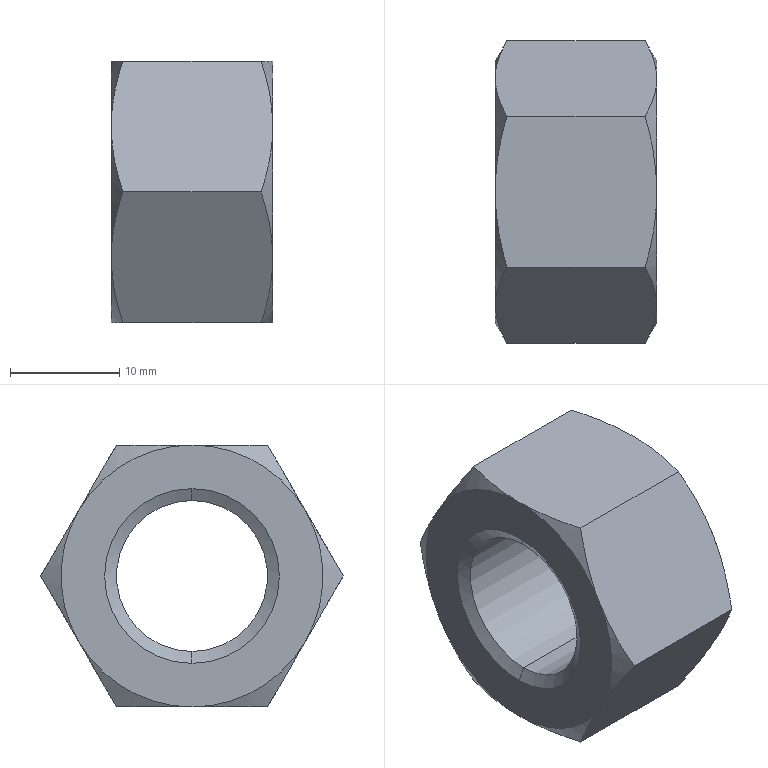Part | SolidWorks | features BaseBody 1 | 1 solid | 26 faces | box 14.8 x 27.713 x 24 mm | volume 5097 mm3 | cone 16 | plane 8 | cylinder 2 | commonest cylinder face diameters 13.835 x2
STEP:
#1=CARTESIAN_POINT('',(0.625,0.,6.918));
#2=VERTEX_POINT('',#1);
#3=CARTESIAN_POINT('',(0.625,0.,-6.918));
#4=VERTEX_POINT('',#3);
#5=CARTESIAN_POINT('',(0.625,0.,0.));
#6=DIRECTION('',(1.,0.,0.));
#7=DIRECTION('',(0.,0.,-1.));
#8=AXIS2_PLACEMENT_3D('',#5,#6,#7);
#9=CIRCLE('',#8,6.918);
#10=EDGE_CURVE('',#2,#4,#9,.T.);
#11=ORIENTED_EDGE('',*,*,#10,.F.);
#12=CARTESIAN_POINT('',(14.175,0.,6.918));
#13=VERTEX_POINT('',#12);
#14=CARTESIAN_POINT('',(-24.735,0.,6.918));
#15=DIRECTION('',(1.,0.,0.));
#16=VECTOR('',#15,1000.);
#17=LINE('',#14,#16);
#18=EDGE_CURVE('',#2,#13,#17,.T.);
#19=ORIENTED_EDGE('',*,*,#18,.T.);
#20=CARTESIAN_POINT('',(14.175,0.,-6.918));
#21=VERTEX_POINT('',#20);
#22=CARTESIAN_POINT('',(14.175,0.,0.));
#23=DIRECTION('',(-1.,0.,0.));
#24=DIRECTION('',(0.,0.,-1.));
#25=AXIS2_PLACEMENT_3D('',#22,#23,#24);
#26=CIRCLE('',#25,6.918);
#27=EDGE_CURVE('',#21,#13,#26,.T.);
#28=ORIENTED_EDGE('',*,*,#27,.F.);
#29=CARTESIAN_POINT('',(-24.735,0.,-6.918));
#30=DIRECTION('',(1.,0.,0.));
#31=VECTOR('',#30,1000.);
#32=LINE('',#29,#31);
#33=EDGE_CURVE('',#4,#21,#32,.T.);
#34=ORIENTED_EDGE('',*,*,#33,.F.);
#35=EDGE_LOOP('',(#11,#19,#28,#34));
#36=FACE_OUTER_BOUND('',#35,.T.);
#37=CARTESIAN_POINT('',(-24.735,0.,0.));
#38=DIRECTION('',(1.,0.,0.));
#39=DIRECTION('',(0.,0.,-1.));
#40=AXIS2_PLACEMENT_3D('',#37,#38,#39);
#41=CYLINDRICAL_SURFACE('',#40,6.918);
#42=ADVANCED_FACE('',(#36),#41,.F.);
#43=ORIENTED_EDGE('',*,*,#10,.T.);
#44=CARTESIAN_POINT('',(0.,0.,-8.));
#45=VERTEX_POINT('',#44);
#46=CARTESIAN_POINT('',(0.,0.,-8.));
#47=DIRECTION('',(-0.5,0.,-0.866));
#48=VECTOR('',#47,1000.);
#49=LINE('',#46,#48);
#50=EDGE_CURVE('',#4,#45,#49,.T.);
#51=ORIENTED_EDGE('',*,*,#50,.T.);
#52=CARTESIAN_POINT('',(0.,0.,8.));
#53=VERTEX_POINT('',#52);
#54=CARTESIAN_POINT('',(0.,0.,0.));
#55=DIRECTION('',(1.,0.,0.));
#56=DIRECTION('',(0.,0.,1.));
#57=AXIS2_PLACEMENT_3D('',#54,#55,#56);
#58=CIRCLE('',#57,8.);
#59=EDGE_CURVE('',#53,#45,#58,.T.);
#60=ORIENTED_EDGE('',*,*,#59,.F.);
#61=CARTESIAN_POINT('',(0.,0.,8.));
#62=DIRECTION('',(-0.5,0.,0.866));
#63=VECTOR('',#62,1000.);
#64=LINE('',#61,#63);
#65=EDGE_CURVE('',#2,#53,#64,.T.);
#66=ORIENTED_EDGE('',*,*,#65,.F.);
#67=EDGE_LOOP('',(#43,#51,#60,#66));
#68=FACE_OUTER_BOUND('',#67,.T.);
#69=CARTESIAN_POINT('',(0.,0.,0.));
#70=DIRECTION('',(-1.,0.,0.));
#71=DIRECTION('',(0.,0.,1.));
#72=AXIS2_PLACEMENT_3D('',#69,#70,#71);
#73=CONICAL_SURFACE('',#72,8.,1.047);
#74=ADVANCED_FACE('',(#68),#73,.F.);
#75=ORIENTED_EDGE('',*,*,#27,.T.);
#76=CARTESIAN_POINT('',(14.8,0.,8.));
#77=VERTEX_POINT('',#76);
#78=CARTESIAN_POINT('',(14.8,0.,8.));
#79=DIRECTION('',(0.5,0.,0.866));
#80=VECTOR('',#79,1000.);
#81=LINE('',#78,#80);
#82=EDGE_CURVE('',#13,#77,#81,.T.);
#83=ORIENTED_EDGE('',*,*,#82,.T.);
#84=CARTESIAN_POINT('',(14.8,0.,-8.));
#85=VERTEX_POINT('',#84);
#86=CARTESIAN_POINT('',(14.8,0.,0.));
#87=DIRECTION('',(-1.,0.,0.));
#88=DIRECTION('',(0.,0.,-1.));
#89=AXIS2_PLACEMENT_3D('',#86,#87,#88);
#90=CIRCLE('',#89,8.);
#91=EDGE_CURVE('',#85,#77,#90,.T.);
#92=ORIENTED_EDGE('',*,*,#91,.F.);
#93=CARTESIAN_POINT('',(14.8,0.,-8.));
#94=DIRECTION('',(0.5,0.,-0.866));
#95=VECTOR('',#94,1000.);
#96=LINE('',#93,#95);
#97=EDGE_CURVE('',#21,#85,#96,.T.);
#98=ORIENTED_EDGE('',*,*,#97,.F.);
#99=EDGE_LOOP('',(#75,#83,#92,#98));
#100=FACE_OUTER_BOUND('',#99,.T.);
#101=CARTESIAN_POINT('',(14.8,0.,0.));
#102=DIRECTION('',(1.,0.,0.));
#103=DIRECTION('',(0.,0.,-1.));
#104=AXIS2_PLACEMENT_3D('',#101,#102,#103);
#105=CONICAL_SURFACE('',#104,8.,1.047);
#106=ADVANCED_FACE('',(#100),#105,.F.);
#107=ORIENTED_EDGE('',*,*,#18,.F.);
#108=CARTESIAN_POINT('',(0.625,0.,0.));
#109=DIRECTION('',(1.,0.,0.));
#110=DIRECTION('',(0.,0.,-1.));
#111=AXIS2_PLACEMENT_3D('',#108,#109,#110);
#112=CIRCLE('',#111,6.918);
#113=EDGE_CURVE('',#4,#2,#112,.T.);
#114=ORIENTED_EDGE('',*,*,#113,.F.);
#115=ORIENTED_EDGE('',*,*,#33,.T.);
#116=CARTESIAN_POINT('',(14.175,0.,0.));
#117=DIRECTION('',(-1.,0.,0.));
#118=DIRECTION('',(0.,0.,-1.));
#119=AXIS2_PLACEMENT_3D('',#116,#117,#118);
#120=CIRCLE('',#119,6.918);
#121=EDGE_CURVE('',#13,#21,#120,.T.);
#122=ORIENTED_EDGE('',*,*,#121,.F.);
#123=EDGE_LOOP('',(#107,#114,#115,#122));
#124=FACE_OUTER_BOUND('',#123,.T.);
#125=CARTESIAN_POINT('',(-24.735,0.,0.));
#126=DIRECTION('',(1.,0.,0.));
#127=DIRECTION('',(0.,0.,-1.));
#128=AXIS2_PLACEMENT_3D('',#125,#126,#127);
#129=CYLINDRICAL_SURFACE('',#128,6.918);
#130=ADVANCED_FACE('',(#124),#129,.F.);
#131=ORIENTED_EDGE('',*,*,#50,.F.);
#132=ORIENTED_EDGE('',*,*,#113,.T.);
#133=ORIENTED_EDGE('',*,*,#65,.T.);
#134=CARTESIAN_POINT('',(0.,0.,0.));
#135=DIRECTION('',(1.,0.,0.));
#136=DIRECTION('',(0.,0.,1.));
#137=AXIS2_PLACEMENT_3D('',#134,#135,#136);
#138=CIRCLE('',#137,8.);
#139=EDGE_CURVE('',#45,#53,#138,.T.);
#140=ORIENTED_EDGE('',*,*,#139,.F.);
#141=EDGE_LOOP('',(#131,#132,#133,#140));
#142=FACE_OUTER_BOUND('',#141,.T.);
#143=CARTESIAN_POINT('',(0.,0.,0.));
#144=DIRECTION('',(-1.,0.,0.));
#145=DIRECTION('',(0.,0.,1.));
#146=AXIS2_PLACEMENT_3D('',#143,#144,#145);
#147=CONICAL_SURFACE('',#146,8.,1.047);
#148=ADVANCED_FACE('',(#142),#147,.F.);
#149=ORIENTED_EDGE('',*,*,#82,.F.);
#150=ORIENTED_EDGE('',*,*,#121,.T.);
#151=ORIENTED_EDGE('',*,*,#97,.T.);
#152=CARTESIAN_POINT('',(14.8,0.,0.));
#153=DIRECTION('',(-1.,0.,0.));
#154=DIRECTION('',(0.,0.,-1.));
#155=AXIS2_PLACEMENT_3D('',#152,#153,#154);
#156=CIRCLE('',#155,8.);
#157=EDGE_CURVE('',#77,#85,#156,.T.);
#158=ORIENTED_EDGE('',*,*,#157,.F.);
#159=EDGE_LOOP('',(#149,#150,#151,#158));
#160=FACE_OUTER_BOUND('',#159,.T.);
#161=CARTESIAN_POINT('',(14.8,0.,0.));
#162=DIRECTION('',(1.,0.,0.));
#163=DIRECTION('',(0.,0.,-1.));
#164=AXIS2_PLACEMENT_3D('',#161,#162,#163);
#165=CONICAL_SURFACE('',#164,8.,1.047);
#166=ADVANCED_FACE('',(#160),#165,.F.);
#167=ORIENTED_EDGE('',*,*,#59,.T.);
#168=ORIENTED_EDGE('',*,*,#139,.T.);
#169=EDGE_LOOP('',(#167,#168));
#170=FACE_BOUND('',#169,.T.);
#171=CARTESIAN_POINT('',(0.,0.,12.));
#172=VERTEX_POINT('',#171);
#173=CARTESIAN_POINT('',(0.,-10.392,6.));
#174=VERTEX_POINT('',#173);
#175=CARTESIAN_POINT('',(0.,0.,0.));
#176=DIRECTION('',(1.,0.,0.));
#177=DIRECTION('',(0.,0.,-1.));
#178=AXIS2_PLACEMENT_3D('',#175,#176,#177);
#179=CIRCLE('',#178,12.);
#180=EDGE_CURVE('',#172,#174,#179,.T.);
#181=ORIENTED_EDGE('',*,*,#180,.F.);
#182=CARTESIAN_POINT('',(0.,10.392,6.));
#183=VERTEX_POINT('',#182);
#184=CARTESIAN_POINT('',(0.,0.,0.));
#185=DIRECTION('',(1.,0.,0.));
#186=DIRECTION('',(0.,0.,-1.));
#187=AXIS2_PLACEMENT_3D('',#184,#185,#186);
#188=CIRCLE('',#187,12.);
#189=EDGE_CURVE('',#183,#172,#188,.T.);
#190=ORIENTED_EDGE('',*,*,#189,.F.);
#191=CARTESIAN_POINT('',(0.,10.392,-6.));
#192=VERTEX_POINT('',#191);
#193=CARTESIAN_POINT('',(0.,0.,0.));
#194=DIRECTION('',(1.,0.,0.));
#195=DIRECTION('',(0.,0.,-1.));
#196=AXIS2_PLACEMENT_3D('',#193,#194,#195);
#197=CIRCLE('',#196,12.);
#198=EDGE_CURVE('',#192,#183,#197,.T.);
#199=ORIENTED_EDGE('',*,*,#198,.F.);
#200=CARTESIAN_POINT('',(0.,0.,-12.));
#201=VERTEX_POINT('',#200);
#202=CARTESIAN_POINT('',(0.,0.,0.));
#203=DIRECTION('',(1.,0.,0.));
#204=DIRECTION('',(0.,0.,-1.));
#205=AXIS2_PLACEMENT_3D('',#202,#203,#204);
#206=CIRCLE('',#205,12.);
#207=EDGE_CURVE('',#201,#192,#206,.T.);
#208=ORIENTED_EDGE('',*,*,#207,.F.);
#209=CARTESIAN_POINT('',(0.,-10.392,-6.));
#210=VERTEX_POINT('',#209);
#211=CARTESIAN_POINT('',(0.,0.,0.));
#212=DIRECTION('',(1.,0.,0.));
#213=DIRECTION('',(0.,0.,-1.));
#214=AXIS2_PLACEMENT_3D('',#211,#212,#213);
#215=CIRCLE('',#214,12.);
#216=EDGE_CURVE('',#210,#201,#215,.T.);
#217=ORIENTED_EDGE('',*,*,#216,.F.);
#218=CARTESIAN_POINT('',(0.,0.,0.));
#219=DIRECTION('',(1.,0.,0.));
#220=DIRECTION('',(0.,0.,-1.));
#221=AXIS2_PLACEMENT_3D('',#218,#219,#220);
#222=CIRCLE('',#221,12.);
#223=EDGE_CURVE('',#174,#210,#222,.T.);
#224=ORIENTED_EDGE('',*,*,#223,.F.);
#225=EDGE_LOOP('',(#181,#190,#199,#208,#217,#224));
#226=FACE_OUTER_BOUND('',#225,.T.);
#227=CARTESIAN_POINT('',(0.,0.,0.));
#228=DIRECTION('',(1.,0.,0.));
#229=DIRECTION('',(0.,0.,-1.));
#230=AXIS2_PLACEMENT_3D('',#227,#228,#229);
#231=PLANE('',#230);
#232=ADVANCED_FACE('',(#170,#226),#231,.F.);
#233=ORIENTED_EDGE('',*,*,#91,.T.);
#234=ORIENTED_EDGE('',*,*,#157,.T.);
#235=EDGE_LOOP('',(#233,#234));
#236=FACE_BOUND('',#235,.T.);
#237=CARTESIAN_POINT('',(14.8,0.,12.));
#238=VERTEX_POINT('',#237);
#239=CARTESIAN_POINT('',(14.8,-10.392,6.));
#240=VERTEX_POINT('',#239);
#241=CARTESIAN_POINT('',(14.8,0.,0.));
#242=DIRECTION('',(1.,0.,0.));
#243=DIRECTION('',(0.,0.,1.));
#244=AXIS2_PLACEMENT_3D('',#241,#242,#243);
#245=CIRCLE('',#244,12.);
#246=EDGE_CURVE('',#238,#240,#245,.T.);
#247=ORIENTED_EDGE('',*,*,#246,.T.);
#248=CARTESIAN_POINT('',(14.8,-10.392,-6.));
#249=VERTEX_POINT('',#248);
#250=CARTESIAN_POINT('',(14.8,0.,0.));
#251=DIRECTION('',(1.,0.,0.));
#252=DIRECTION('',(0.,0.,1.));
#253=AXIS2_PLACEMENT_3D('',#250,#251,#252);
#254=CIRCLE('',#253,12.);
#255=EDGE_CURVE('',#240,#249,#254,.T.);
#256=ORIENTED_EDGE('',*,*,#255,.T.);
#257=CARTESIAN_POINT('',(14.8,0.,-12.));
#258=VERTEX_POINT('',#257);
#259=CARTESIAN_POINT('',(14.8,0.,0.));
#260=DIRECTION('',(1.,0.,0.));
#261=DIRECTION('',(0.,0.,1.));
#262=AXIS2_PLACEMENT_3D('',#259,#260,#261);
#263=CIRCLE('',#262,12.);
#264=EDGE_CURVE('',#249,#258,#263,.T.);
#265=ORIENTED_EDGE('',*,*,#264,.T.);
#266=CARTESIAN_POINT('',(14.8,10.392,-6.));
#267=VERTEX_POINT('',#266);
#268=CARTESIAN_POINT('',(14.8,0.,0.));
#269=DIRECTION('',(1.,0.,0.));
#270=DIRECTION('',(0.,0.,1.));
#271=AXIS2_PLACEMENT_3D('',#268,#269,#270);
#272=CIRCLE('',#271,12.);
#273=EDGE_CURVE('',#258,#267,#272,.T.);
#274=ORIENTED_EDGE('',*,*,#273,.T.);
#275=CARTESIAN_POINT('',(14.8,10.392,6.));
#276=VERTEX_POINT('',#275);
#277=CARTESIAN_POINT('',(14.8,0.,0.));
#278=DIRECTION('',(1.,0.,0.));
#279=DIRECTION('',(0.,0.,1.));
#280=AXIS2_PLACEMENT_3D('',#277,#278,#279);
#281=CIRCLE('',#280,12.);
#282=EDGE_CURVE('',#267,#276,#281,.T.);
#283=ORIENTED_EDGE('',*,*,#282,.T.);
#284=CARTESIAN_POINT('',(14.8,0.,0.));
#285=DIRECTION('',(1.,0.,0.));
#286=DIRECTION('',(0.,0.,1.));
#287=AXIS2_PLACEMENT_3D('',#284,#285,#286);
#288=CIRCLE('',#287,12.);
#289=EDGE_CURVE('',#276,#238,#288,.T.);
#290=ORIENTED_EDGE('',*,*,#289,.T.);
#291=EDGE_LOOP('',(#247,#256,#265,#274,#283,#290));
#292=FACE_OUTER_BOUND('',#291,.T.);
#293=CARTESIAN_POINT('',(14.8,0.,0.));
#294=DIRECTION('',(1.,0.,0.));
#295=DIRECTION('',(0.,0.,-1.));
#296=AXIS2_PLACEMENT_3D('',#293,#294,#295);
#297=PLANE('',#296);
#298=ADVANCED_FACE('',(#236,#292),#297,.T.);
#299=ORIENTED_EDGE('',*,*,#223,.T.);
#300=CARTESIAN_POINT('',(1.072,-13.856,0.000000014));
#301=VERTEX_POINT('',#300);
#302=CARTESIAN_POINT('',(0.,-10.392,-6.));
#303=CARTESIAN_POINT('',(0.,-10.983,-4.976));
#304=CARTESIAN_POINT('',(0.1025,-11.567,-3.966));
#305=CARTESIAN_POINT('',(0.4756,-12.72,-1.968));
#306=CARTESIAN_POINT('',(0.7451,-13.291,-0.9802));
#307=CARTESIAN_POINT('',(1.072,-13.856,0.000000014));
#308=B_SPLINE_CURVE_WITH_KNOTS('',3,(#302,#303,#304,#305,#306,#307),.UNSPECIFIED.,.F.,.F.,(4,2,4),(0.,0.003505,0.007011),.UNSPECIFIED.);
#309=EDGE_CURVE('',#210,#301,#308,.T.);
#310=ORIENTED_EDGE('',*,*,#309,.T.);
#311=CARTESIAN_POINT('',(1.072,-13.856,0.000000014));
#312=CARTESIAN_POINT('',(0.7451,-13.291,0.9802));
#313=CARTESIAN_POINT('',(0.4756,-12.72,1.968));
#314=CARTESIAN_POINT('',(0.1025,-11.567,3.966));
#315=CARTESIAN_POINT('',(0.,-10.983,4.976));
#316=CARTESIAN_POINT('',(0.,-10.392,6.));
#317=B_SPLINE_CURVE_WITH_KNOTS('',3,(#311,#312,#313,#314,#315,#316),.UNSPECIFIED.,.F.,.F.,(4,2,4),(0.,0.003505,0.007011),.UNSPECIFIED.);
#318=EDGE_CURVE('',#301,#174,#317,.T.);
#319=ORIENTED_EDGE('',*,*,#318,.T.);
#320=EDGE_LOOP('',(#299,#310,#319));
#321=FACE_OUTER_BOUND('',#320,.T.);
#322=CARTESIAN_POINT('',(1.078,0.,0.));
#323=DIRECTION('',(1.,0.,0.));
#324=DIRECTION('',(0.,0.,-1.));
#325=AXIS2_PLACEMENT_3D('',#322,#323,#324);
#326=CONICAL_SURFACE('',#325,13.868,1.047);
#327=ADVANCED_FACE('',(#321),#326,.T.);
#328=ORIENTED_EDGE('',*,*,#180,.T.);
#329=CARTESIAN_POINT('',(1.072,-6.928,12.));
#330=VERTEX_POINT('',#329);
#331=CARTESIAN_POINT('',(0.,-10.392,6.));
#332=CARTESIAN_POINT('',(0.,-9.801,7.024));
#333=CARTESIAN_POINT('',(0.1025,-9.218,8.034));
#334=CARTESIAN_POINT('',(0.4756,-8.064,10.032));
#335=CARTESIAN_POINT('',(0.7451,-7.494,11.02));
#336=CARTESIAN_POINT('',(1.072,-6.928,12.));
#337=B_SPLINE_CURVE_WITH_KNOTS('',3,(#331,#332,#333,#334,#335,#336),.UNSPECIFIED.,.F.,.F.,(4,2,4),(0.,0.003505,0.007011),.UNSPECIFIED.);
#338=EDGE_CURVE('',#174,#330,#337,.T.);
#339=ORIENTED_EDGE('',*,*,#338,.T.);
#340=CARTESIAN_POINT('',(1.072,-6.928,12.));
#341=CARTESIAN_POINT('',(0.7451,-5.796,12.));
#342=CARTESIAN_POINT('',(0.4756,-4.656,12.));
#343=CARTESIAN_POINT('',(0.1025,-2.349,12.));
#344=CARTESIAN_POINT('',(0.,-1.182,12.));
#345=CARTESIAN_POINT('',(0.,0.,12.));
#346=B_SPLINE_CURVE_WITH_KNOTS('',3,(#340,#341,#342,#343,#344,#345),.UNSPECIFIED.,.F.,.F.,(4,2,4),(0.,0.003505,0.007011),.UNSPECIFIED.);
#347=EDGE_CURVE('',#330,#172,#346,.T.);
#348=ORIENTED_EDGE('',*,*,#347,.T.);
#349=EDGE_LOOP('',(#328,#339,#348));
#350=FACE_OUTER_BOUND('',#349,.T.);
#351=CARTESIAN_POINT('',(1.078,0.,0.));
#352=DIRECTION('',(1.,0.,0.));
#353=DIRECTION('',(0.,0.,-1.));
#354=AXIS2_PLACEMENT_3D('',#351,#352,#353);
#355=CONICAL_SURFACE('',#354,13.868,1.047);
#356=ADVANCED_FACE('',(#350),#355,.T.);
#357=ORIENTED_EDGE('',*,*,#189,.T.);
#358=CARTESIAN_POINT('',(1.072,6.928,12.));
#359=VERTEX_POINT('',#358);
#360=CARTESIAN_POINT('',(0.,0.,12.));
#361=CARTESIAN_POINT('',(0.,1.182,12.));
#362=CARTESIAN_POINT('',(0.1025,2.349,12.));
#363=CARTESIAN_POINT('',(0.4756,4.656,12.));
#364=CARTESIAN_POINT('',(0.7451,5.796,12.));
#365=CARTESIAN_POINT('',(1.072,6.928,12.));
#366=B_SPLINE_CURVE_WITH_KNOTS('',3,(#360,#361,#362,#363,#364,#365),.UNSPECIFIED.,.F.,.F.,(4,2,4),(0.,0.003505,0.007011),.UNSPECIFIED.);
#367=EDGE_CURVE('',#172,#359,#366,.T.);
#368=ORIENTED_EDGE('',*,*,#367,.T.);
#369=CARTESIAN_POINT('',(1.072,6.928,12.));
#370=CARTESIAN_POINT('',(0.7451,7.494,11.02));
#371=CARTESIAN_POINT('',(0.4756,8.064,10.032));
#372=CARTESIAN_POINT('',(0.1025,9.218,8.034));
#373=CARTESIAN_POINT('',(0.,9.801,7.024));
#374=CARTESIAN_POINT('',(0.,10.392,6.));
#375=B_SPLINE_CURVE_WITH_KNOTS('',3,(#369,#370,#371,#372,#373,#374),.UNSPECIFIED.,.F.,.F.,(4,2,4),(0.,0.003505,0.007011),.UNSPECIFIED.);
#376=EDGE_CURVE('',#359,#183,#375,.T.);
#377=ORIENTED_EDGE('',*,*,#376,.T.);
#378=EDGE_LOOP('',(#357,#368,#377));
#379=FACE_OUTER_BOUND('',#378,.T.);
#380=CARTESIAN_POINT('',(1.078,0.,0.));
#381=DIRECTION('',(1.,0.,0.));
#382=DIRECTION('',(0.,0.,-1.));
#383=AXIS2_PLACEMENT_3D('',#380,#381,#382);
#384=CONICAL_SURFACE('',#383,13.868,1.047);
#385=ADVANCED_FACE('',(#379),#384,.T.);
#386=ORIENTED_EDGE('',*,*,#198,.T.);
#387=CARTESIAN_POINT('',(1.072,13.856,-0.000000014));
#388=VERTEX_POINT('',#387);
#389=CARTESIAN_POINT('',(0.,10.392,6.));
#390=CARTESIAN_POINT('',(0.,10.983,4.976));
#391=CARTESIAN_POINT('',(0.1025,11.567,3.966));
#392=CARTESIAN_POINT('',(0.4756,12.72,1.968));
#393=CARTESIAN_POINT('',(0.7451,13.291,0.9802));
#394=CARTESIAN_POINT('',(1.072,13.856,-0.000000014));
#395=B_SPLINE_CURVE_WITH_KNOTS('',3,(#389,#390,#391,#392,#393,#394),.UNSPECIFIED.,.F.,.F.,(4,2,4),(0.,0.003505,0.007011),.UNSPECIFIED.);
#396=EDGE_CURVE('',#183,#388,#395,.T.);
#397=ORIENTED_EDGE('',*,*,#396,.T.);
#398=CARTESIAN_POINT('',(1.072,13.856,-0.000000014));
#399=CARTESIAN_POINT('',(0.7451,13.291,-0.9802));
#400=CARTESIAN_POINT('',(0.4756,12.72,-1.968));
#401=CARTESIAN_POINT('',(0.1025,11.567,-3.966));
#402=CARTESIAN_POINT('',(0.,10.983,-4.976));
#403=CARTESIAN_POINT('',(0.,10.392,-6.));
#404=B_SPLINE_CURVE_WITH_KNOTS('',3,(#398,#399,#400,#401,#402,#403),.UNSPECIFIED.,.F.,.F.,(4,2,4),(0.,0.003505,0.007011),.UNSPECIFIED.);
#405=EDGE_CURVE('',#388,#192,#404,.T.);
#406=ORIENTED_EDGE('',*,*,#405,.T.);
#407=EDGE_LOOP('',(#386,#397,#406));
#408=FACE_OUTER_BOUND('',#407,.T.);
#409=CARTESIAN_POINT('',(1.078,0.,0.));
#410=DIRECTION('',(1.,0.,0.));
#411=DIRECTION('',(0.,0.,-1.));
#412=AXIS2_PLACEMENT_3D('',#409,#410,#411);
#413=CONICAL_SURFACE('',#412,13.868,1.047);
#414=ADVANCED_FACE('',(#408),#413,.T.);
#415=CARTESIAN_POINT('',(1.072,6.928,-12.));
#416=VERTEX_POINT('',#415);
#417=CARTESIAN_POINT('',(1.072,6.928,-12.));
#418=CARTESIAN_POINT('',(0.7451,5.796,-12.));
#419=CARTESIAN_POINT('',(0.4756,4.656,-12.));
#420=CARTESIAN_POINT('',(0.1025,2.349,-12.));
#421=CARTESIAN_POINT('',(0.,1.182,-12.));
#422=CARTESIAN_POINT('',(0.,0.,-12.));
#423=B_SPLINE_CURVE_WITH_KNOTS('',3,(#417,#418,#419,#420,#421,#422),.UNSPECIFIED.,.F.,.F.,(4,2,4),(0.,0.003505,0.007011),.UNSPECIFIED.);
#424=EDGE_CURVE('',#416,#201,#423,.T.);
#425=ORIENTED_EDGE('',*,*,#424,.T.);
#426=ORIENTED_EDGE('',*,*,#207,.T.);
#427=CARTESIAN_POINT('',(0.,10.392,-6.));
#428=CARTESIAN_POINT('',(0.,9.801,-7.024));
#429=CARTESIAN_POINT('',(0.1025,9.218,-8.034));
#430=CARTESIAN_POINT('',(0.4756,8.064,-10.032));
#431=CARTESIAN_POINT('',(0.7451,7.494,-11.02));
#432=CARTESIAN_POINT('',(1.072,6.928,-12.));
#433=B_SPLINE_CURVE_WITH_KNOTS('',3,(#427,#428,#429,#430,#431,#432),.UNSPECIFIED.,.F.,.F.,(4,2,4),(0.,0.003505,0.007011),.UNSPECIFIED.);
#434=EDGE_CURVE('',#192,#416,#433,.T.);
#435=ORIENTED_EDGE('',*,*,#434,.T.);
#436=EDGE_LOOP('',(#425,#426,#435));
#437=FACE_OUTER_BOUND('',#436,.T.);
#438=CARTESIAN_POINT('',(1.078,0.,0.));
#439=DIRECTION('',(1.,0.,0.));
#440=DIRECTION('',(0.,0.,-1.));
#441=AXIS2_PLACEMENT_3D('',#438,#439,#440);
#442=CONICAL_SURFACE('',#441,13.868,1.047);
#443=ADVANCED_FACE('',(#437),#442,.T.);
#444=CARTESIAN_POINT('',(1.072,-6.928,-12.));
#445=VERTEX_POINT('',#444);
#446=CARTESIAN_POINT('',(1.072,-6.928,-12.));
#447=CARTESIAN_POINT('',(0.7451,-7.494,-11.02));
#448=CARTESIAN_POINT('',(0.4756,-8.064,-10.032));
#449=CARTESIAN_POINT('',(0.1025,-9.218,-8.034));
#450=CARTESIAN_POINT('',(0.,-9.801,-7.024));
#451=CARTESIAN_POINT('',(0.,-10.392,-6.));
#452=B_SPLINE_CURVE_WITH_KNOTS('',3,(#446,#447,#448,#449,#450,#451),.UNSPECIFIED.,.F.,.F.,(4,2,4),(0.,0.003505,0.007011),.UNSPECIFIED.);
#453=EDGE_CURVE('',#445,#210,#452,.T.);
#454=ORIENTED_EDGE('',*,*,#453,.T.);
#455=ORIENTED_EDGE('',*,*,#216,.T.);
#456=CARTESIAN_POINT('',(0.,0.,-12.));
#457=CARTESIAN_POINT('',(0.,-1.182,-12.));
#458=CARTESIAN_POINT('',(0.1025,-2.349,-12.));
#459=CARTESIAN_POINT('',(0.4756,-4.656,-12.));
#460=CARTESIAN_POINT('',(0.7451,-5.796,-12.));
#461=CARTESIAN_POINT('',(1.072,-6.928,-12.));
#462=B_SPLINE_CURVE_WITH_KNOTS('',3,(#456,#457,#458,#459,#460,#461),.UNSPECIFIED.,.F.,.F.,(4,2,4),(0.,0.003505,0.007011),.UNSPECIFIED.);
#463=EDGE_CURVE('',#201,#445,#462,.T.);
#464=ORIENTED_EDGE('',*,*,#463,.T.);
#465=EDGE_LOOP('',(#454,#455,#464));
#466=FACE_OUTER_BOUND('',#465,.T.);
#467=CARTESIAN_POINT('',(1.078,0.,0.));
#468=DIRECTION('',(1.,0.,0.));
#469=DIRECTION('',(0.,0.,-1.));
#470=AXIS2_PLACEMENT_3D('',#467,#468,#469);
#471=CONICAL_SURFACE('',#470,13.868,1.047);
#472=ADVANCED_FACE('',(#466),#471,.T.);
#473=CARTESIAN_POINT('',(13.728,-13.856,0.000000038));
#474=VERTEX_POINT('',#473);
#475=CARTESIAN_POINT('',(13.728,-13.856,0.000000038));
#476=CARTESIAN_POINT('',(14.055,-13.291,-0.9802));
#477=CARTESIAN_POINT('',(14.324,-12.72,-1.968));
#478=CARTESIAN_POINT('',(14.698,-11.567,-3.966));
#479=CARTESIAN_POINT('',(14.8,-10.983,-4.976));
#480=CARTESIAN_POINT('',(14.8,-10.392,-6.));
#481=B_SPLINE_CURVE_WITH_KNOTS('',3,(#475,#476,#477,#478,#479,#480),.UNSPECIFIED.,.F.,.F.,(4,2,4),(0.,0.003505,0.007011),.UNSPECIFIED.);
#482=EDGE_CURVE('',#474,#249,#481,.T.);
#483=ORIENTED_EDGE('',*,*,#482,.T.);
#484=ORIENTED_EDGE('',*,*,#255,.F.);
#485=CARTESIAN_POINT('',(14.8,-10.392,6.));
#486=CARTESIAN_POINT('',(14.8,-10.983,4.976));
#487=CARTESIAN_POINT('',(14.698,-11.567,3.966));
#488=CARTESIAN_POINT('',(14.324,-12.72,1.968));
#489=CARTESIAN_POINT('',(14.055,-13.291,0.9802));
#490=CARTESIAN_POINT('',(13.728,-13.856,0.000000038));
#491=B_SPLINE_CURVE_WITH_KNOTS('',3,(#485,#486,#487,#488,#489,#490),.UNSPECIFIED.,.F.,.F.,(4,2,4),(0.,0.003505,0.007011),.UNSPECIFIED.);
#492=EDGE_CURVE('',#240,#474,#491,.T.);
#493=ORIENTED_EDGE('',*,*,#492,.T.);
#494=EDGE_LOOP('',(#483,#484,#493));
#495=FACE_OUTER_BOUND('',#494,.T.);
#496=CARTESIAN_POINT('',(13.722,0.,0.));
#497=DIRECTION('',(-1.,0.,0.));
#498=DIRECTION('',(0.,0.,1.));
#499=AXIS2_PLACEMENT_3D('',#496,#497,#498);
#500=CONICAL_SURFACE('',#499,13.868,1.047);
#501=ADVANCED_FACE('',(#495),#500,.T.);
#502=CARTESIAN_POINT('',(13.728,-6.928,12.));
#503=VERTEX_POINT('',#502);
#504=CARTESIAN_POINT('',(13.728,-6.928,12.));
#505=CARTESIAN_POINT('',(14.055,-7.494,11.02));
#506=CARTESIAN_POINT('',(14.324,-8.064,10.032));
#507=CARTESIAN_POINT('',(14.698,-9.218,8.034));
#508=CARTESIAN_POINT('',(14.8,-9.801,7.024));
#509=CARTESIAN_POINT('',(14.8,-10.392,6.));
#510=B_SPLINE_CURVE_WITH_KNOTS('',3,(#504,#505,#506,#507,#508,#509),.UNSPECIFIED.,.F.,.F.,(4,2,4),(0.,0.003505,0.007011),.UNSPECIFIED.);
#511=EDGE_CURVE('',#503,#240,#510,.T.);
#512=ORIENTED_EDGE('',*,*,#511,.T.);
#513=ORIENTED_EDGE('',*,*,#246,.F.);
#514=CARTESIAN_POINT('',(14.8,0.,12.));
#515=CARTESIAN_POINT('',(14.8,-1.182,12.));
#516=CARTESIAN_POINT('',(14.698,-2.349,12.));
#517=CARTESIAN_POINT('',(14.324,-4.656,12.));
#518=CARTESIAN_POINT('',(14.055,-5.796,12.));
#519=CARTESIAN_POINT('',(13.728,-6.928,12.));
#520=B_SPLINE_CURVE_WITH_KNOTS('',3,(#514,#515,#516,#517,#518,#519),.UNSPECIFIED.,.F.,.F.,(4,2,4),(0.,0.003505,0.007011),.UNSPECIFIED.);
#521=EDGE_CURVE('',#238,#503,#520,.T.);
#522=ORIENTED_EDGE('',*,*,#521,.T.);
#523=EDGE_LOOP('',(#512,#513,#522));
#524=FACE_OUTER_BOUND('',#523,.T.);
#525=CARTESIAN_POINT('',(13.722,0.,0.));
#526=DIRECTION('',(-1.,0.,0.));
#527=DIRECTION('',(0.,0.,1.));
#528=AXIS2_PLACEMENT_3D('',#525,#526,#527);
#529=CONICAL_SURFACE('',#528,13.868,1.047);
#530=ADVANCED_FACE('',(#524),#529,.T.);
#531=CARTESIAN_POINT('',(13.728,6.928,12.));
#532=VERTEX_POINT('',#531);
#533=CARTESIAN_POINT('',(13.728,6.928,12.));
#534=CARTESIAN_POINT('',(14.055,5.796,12.));
#535=CARTESIAN_POINT('',(14.324,4.656,12.));
#536=CARTESIAN_POINT('',(14.698,2.349,12.));
#537=CARTESIAN_POINT('',(14.8,1.182,12.));
#538=CARTESIAN_POINT('',(14.8,0.,12.));
#539=B_SPLINE_CURVE_WITH_KNOTS('',3,(#533,#534,#535,#536,#537,#538),.UNSPECIFIED.,.F.,.F.,(4,2,4),(0.,0.003505,0.007011),.UNSPECIFIED.);
#540=EDGE_CURVE('',#532,#238,#539,.T.);
#541=ORIENTED_EDGE('',*,*,#540,.T.);
#542=ORIENTED_EDGE('',*,*,#289,.F.);
#543=CARTESIAN_POINT('',(14.8,10.392,6.));
#544=CARTESIAN_POINT('',(14.8,9.801,7.024));
#545=CARTESIAN_POINT('',(14.698,9.218,8.034));
#546=CARTESIAN_POINT('',(14.324,8.064,10.032));
#547=CARTESIAN_POINT('',(14.055,7.494,11.02));
#548=CARTESIAN_POINT('',(13.728,6.928,12.));
#549=B_SPLINE_CURVE_WITH_KNOTS('',3,(#543,#544,#545,#546,#547,#548),.UNSPECIFIED.,.F.,.F.,(4,2,4),(0.,0.003505,0.007011),.UNSPECIFIED.);
#550=EDGE_CURVE('',#276,#532,#549,.T.);
#551=ORIENTED_EDGE('',*,*,#550,.T.);
#552=EDGE_LOOP('',(#541,#542,#551));
#553=FACE_OUTER_BOUND('',#552,.T.);
#554=CARTESIAN_POINT('',(13.722,0.,0.));
#555=DIRECTION('',(-1.,0.,0.));
#556=DIRECTION('',(0.,0.,1.));
#557=AXIS2_PLACEMENT_3D('',#554,#555,#556);
#558=CONICAL_SURFACE('',#557,13.868,1.047);
#559=ADVANCED_FACE('',(#553),#558,.T.);
#560=ORIENTED_EDGE('',*,*,#282,.F.);
#561=CARTESIAN_POINT('',(13.728,13.856,0.000000014));
#562=VERTEX_POINT('',#561);
#563=CARTESIAN_POINT('',(14.8,10.392,-6.));
#564=CARTESIAN_POINT('',(14.8,10.983,-4.976));
#565=CARTESIAN_POINT('',(14.698,11.567,-3.966));
#566=CARTESIAN_POINT('',(14.324,12.72,-1.968));
#567=CARTESIAN_POINT('',(14.055,13.291,-0.9802));
#568=CARTESIAN_POINT('',(13.728,13.856,0.000000014));
#569=B_SPLINE_CURVE_WITH_KNOTS('',3,(#563,#564,#565,#566,#567,#568),.UNSPECIFIED.,.F.,.F.,(4,2,4),(0.,0.003505,0.007011),.UNSPECIFIED.);
#570=EDGE_CURVE('',#267,#562,#569,.T.);
#571=ORIENTED_EDGE('',*,*,#570,.T.);
#572=CARTESIAN_POINT('',(13.728,13.856,0.000000014));
#573=CARTESIAN_POINT('',(14.055,13.291,0.9802));
#574=CARTESIAN_POINT('',(14.324,12.72,1.968));
#575=CARTESIAN_POINT('',(14.698,11.567,3.966));
#576=CARTESIAN_POINT('',(14.8,10.983,4.976));
#577=CARTESIAN_POINT('',(14.8,10.392,6.));
#578=B_SPLINE_CURVE_WITH_KNOTS('',3,(#572,#573,#574,#575,#576,#577),.UNSPECIFIED.,.F.,.F.,(4,2,4),(0.,0.003505,0.007011),.UNSPECIFIED.);
#579=EDGE_CURVE('',#562,#276,#578,.T.);
#580=ORIENTED_EDGE('',*,*,#579,.T.);
#581=EDGE_LOOP('',(#560,#571,#580));
#582=FACE_OUTER_BOUND('',#581,.T.);
#583=CARTESIAN_POINT('',(13.722,0.,0.));
#584=DIRECTION('',(-1.,0.,0.));
#585=DIRECTION('',(0.,0.,1.));
#586=AXIS2_PLACEMENT_3D('',#583,#584,#585);
#587=CONICAL_SURFACE('',#586,13.868,1.047);
#588=ADVANCED_FACE('',(#582),#587,.T.);
#589=ORIENTED_EDGE('',*,*,#273,.F.);
#590=CARTESIAN_POINT('',(13.728,6.928,-12.));
#591=VERTEX_POINT('',#590);
#592=CARTESIAN_POINT('',(14.8,0.,-12.));
#593=CARTESIAN_POINT('',(14.8,1.182,-12.));
#594=CARTESIAN_POINT('',(14.698,2.349,-12.));
#595=CARTESIAN_POINT('',(14.324,4.656,-12.));
#596=CARTESIAN_POINT('',(14.055,5.796,-12.));
#597=CARTESIAN_POINT('',(13.728,6.928,-12.));
#598=B_SPLINE_CURVE_WITH_KNOTS('',3,(#592,#593,#594,#595,#596,#597),.UNSPECIFIED.,.F.,.F.,(4,2,4),(0.,0.003505,0.007011),.UNSPECIFIED.);
#599=EDGE_CURVE('',#258,#591,#598,.T.);
#600=ORIENTED_EDGE('',*,*,#599,.T.);
#601=CARTESIAN_POINT('',(13.728,6.928,-12.));
#602=CARTESIAN_POINT('',(14.055,7.494,-11.02));
#603=CARTESIAN_POINT('',(14.324,8.064,-10.032));
#604=CARTESIAN_POINT('',(14.698,9.218,-8.034));
#605=CARTESIAN_POINT('',(14.8,9.801,-7.024));
#606=CARTESIAN_POINT('',(14.8,10.392,-6.));
#607=B_SPLINE_CURVE_WITH_KNOTS('',3,(#601,#602,#603,#604,#605,#606),.UNSPECIFIED.,.F.,.F.,(4,2,4),(0.,0.003505,0.007011),.UNSPECIFIED.);
#608=EDGE_CURVE('',#591,#267,#607,.T.);
#609=ORIENTED_EDGE('',*,*,#608,.T.);
#610=EDGE_LOOP('',(#589,#600,#609));
#611=FACE_OUTER_BOUND('',#610,.T.);
#612=CARTESIAN_POINT('',(13.722,0.,0.));
#613=DIRECTION('',(-1.,0.,0.));
#614=DIRECTION('',(0.,0.,1.));
#615=AXIS2_PLACEMENT_3D('',#612,#613,#614);
#616=CONICAL_SURFACE('',#615,13.868,1.047);
#617=ADVANCED_FACE('',(#611),#616,.T.);
#618=ORIENTED_EDGE('',*,*,#264,.F.);
#619=CARTESIAN_POINT('',(13.728,-6.928,-12.));
#620=VERTEX_POINT('',#619);
#621=CARTESIAN_POINT('',(14.8,-10.392,-6.));
#622=CARTESIAN_POINT('',(14.8,-9.801,-7.024));
#623=CARTESIAN_POINT('',(14.698,-9.218,-8.034));
#624=CARTESIAN_POINT('',(14.324,-8.064,-10.032));
#625=CARTESIAN_POINT('',(14.055,-7.494,-11.02));
#626=CARTESIAN_POINT('',(13.728,-6.928,-12.));
#627=B_SPLINE_CURVE_WITH_KNOTS('',3,(#621,#622,#623,#624,#625,#626),.UNSPECIFIED.,.F.,.F.,(4,2,4),(0.,0.003505,0.007011),.UNSPECIFIED.);
#628=EDGE_CURVE('',#249,#620,#627,.T.);
#629=ORIENTED_EDGE('',*,*,#628,.T.);
#630=CARTESIAN_POINT('',(13.728,-6.928,-12.));
#631=CARTESIAN_POINT('',(14.055,-5.796,-12.));
#632=CARTESIAN_POINT('',(14.324,-4.656,-12.));
#633=CARTESIAN_POINT('',(14.698,-2.349,-12.));
#634=CARTESIAN_POINT('',(14.8,-1.182,-12.));
#635=CARTESIAN_POINT('',(14.8,0.,-12.));
#636=B_SPLINE_CURVE_WITH_KNOTS('',3,(#630,#631,#632,#633,#634,#635),.UNSPECIFIED.,.F.,.F.,(4,2,4),(0.,0.003505,0.007011),.UNSPECIFIED.);
#637=EDGE_CURVE('',#620,#258,#636,.T.);
#638=ORIENTED_EDGE('',*,*,#637,.T.);
#639=EDGE_LOOP('',(#618,#629,#638));
#640=FACE_OUTER_BOUND('',#639,.T.);
#641=CARTESIAN_POINT('',(13.722,0.,0.));
#642=DIRECTION('',(-1.,0.,0.));
#643=DIRECTION('',(0.,0.,1.));
#644=AXIS2_PLACEMENT_3D('',#641,#642,#643);
#645=CONICAL_SURFACE('',#644,13.868,1.047);
#646=ADVANCED_FACE('',(#640),#645,.T.);
#647=CARTESIAN_POINT('',(0.,-13.856,0.));
#648=DIRECTION('',(-1.,0.,0.));
#649=VECTOR('',#648,1000.);
#650=LINE('',#647,#649);
#651=EDGE_CURVE('',#474,#301,#650,.T.);
#652=ORIENTED_EDGE('',*,*,#651,.T.);
#653=ORIENTED_EDGE('',*,*,#309,.F.);
#654=ORIENTED_EDGE('',*,*,#453,.F.);
#655=CARTESIAN_POINT('',(0.,-6.928,-12.));
#656=DIRECTION('',(1.,0.,0.));
#657=VECTOR('',#656,1000.);
#658=LINE('',#655,#657);
#659=EDGE_CURVE('',#445,#620,#658,.T.);
#660=ORIENTED_EDGE('',*,*,#659,.T.);
#661=ORIENTED_EDGE('',*,*,#628,.F.);
#662=ORIENTED_EDGE('',*,*,#482,.F.);
#663=EDGE_LOOP('',(#652,#653,#654,#660,#661,#662));
#664=FACE_OUTER_BOUND('',#663,.T.);
#665=CARTESIAN_POINT('',(0.,-6.928,-12.));
#666=DIRECTION('',(0.,-0.866,-0.5));
#667=DIRECTION('',(0.,0.5,-0.866));
#668=AXIS2_PLACEMENT_3D('',#665,#666,#667);
#669=PLANE('',#668);
#670=ADVANCED_FACE('',(#664),#669,.T.);
#671=ORIENTED_EDGE('',*,*,#511,.F.);
#672=CARTESIAN_POINT('',(0.,-6.928,12.));
#673=DIRECTION('',(-1.,0.,0.));
#674=VECTOR('',#673,1000.);
#675=LINE('',#672,#674);
#676=EDGE_CURVE('',#503,#330,#675,.T.);
#677=ORIENTED_EDGE('',*,*,#676,.T.);
#678=ORIENTED_EDGE('',*,*,#338,.F.);
#679=ORIENTED_EDGE('',*,*,#318,.F.);
#680=ORIENTED_EDGE('',*,*,#651,.F.);
#681=ORIENTED_EDGE('',*,*,#492,.F.);
#682=EDGE_LOOP('',(#671,#677,#678,#679,#680,#681));
#683=FACE_OUTER_BOUND('',#682,.T.);
#684=CARTESIAN_POINT('',(0.,-13.856,0.));
#685=DIRECTION('',(0.,-0.866,0.5));
#686=DIRECTION('',(0.,-0.5,-0.866));
#687=AXIS2_PLACEMENT_3D('',#684,#685,#686);
#688=PLANE('',#687);
#689=ADVANCED_FACE('',(#683),#688,.T.);
#690=ORIENTED_EDGE('',*,*,#540,.F.);
#691=CARTESIAN_POINT('',(0.,6.928,12.));
#692=DIRECTION('',(-1.,0.,0.));
#693=VECTOR('',#692,1000.);
#694=LINE('',#691,#693);
#695=EDGE_CURVE('',#532,#359,#694,.T.);
#696=ORIENTED_EDGE('',*,*,#695,.T.);
#697=ORIENTED_EDGE('',*,*,#367,.F.);
#698=ORIENTED_EDGE('',*,*,#347,.F.);
#699=ORIENTED_EDGE('',*,*,#676,.F.);
#700=ORIENTED_EDGE('',*,*,#521,.F.);
#701=EDGE_LOOP('',(#690,#696,#697,#698,#699,#700));
#702=FACE_OUTER_BOUND('',#701,.T.);
#703=CARTESIAN_POINT('',(0.,-6.928,12.));
#704=DIRECTION('',(0.,0.,1.));
#705=DIRECTION('',(1.,0.,0.));
#706=AXIS2_PLACEMENT_3D('',#703,#704,#705);
#707=PLANE('',#706);
#708=ADVANCED_FACE('',(#702),#707,.T.);
#709=ORIENTED_EDGE('',*,*,#579,.F.);
#710=CARTESIAN_POINT('',(0.,13.856,0.));
#711=DIRECTION('',(-1.,0.,0.));
#712=VECTOR('',#711,1000.);
#713=LINE('',#710,#712);
#714=EDGE_CURVE('',#562,#388,#713,.T.);
#715=ORIENTED_EDGE('',*,*,#714,.T.);
#716=ORIENTED_EDGE('',*,*,#396,.F.);
#717=ORIENTED_EDGE('',*,*,#376,.F.);
#718=ORIENTED_EDGE('',*,*,#695,.F.);
#719=ORIENTED_EDGE('',*,*,#550,.F.);
#720=EDGE_LOOP('',(#709,#715,#716,#717,#718,#719));
#721=FACE_OUTER_BOUND('',#720,.T.);
#722=CARTESIAN_POINT('',(0.,6.928,12.));
#723=DIRECTION('',(0.,0.866,0.5));
#724=DIRECTION('',(0.,-0.5,0.866));
#725=AXIS2_PLACEMENT_3D('',#722,#723,#724);
#726=PLANE('',#725);
#727=ADVANCED_FACE('',(#721),#726,.T.);
#728=CARTESIAN_POINT('',(0.,6.928,-12.));
#729=DIRECTION('',(-1.,0.,0.));
#730=VECTOR('',#729,1000.);
#731=LINE('',#728,#730);
#732=EDGE_CURVE('',#591,#416,#731,.T.);
#733=ORIENTED_EDGE('',*,*,#732,.T.);
#734=ORIENTED_EDGE('',*,*,#434,.F.);
#735=ORIENTED_EDGE('',*,*,#405,.F.);
#736=ORIENTED_EDGE('',*,*,#714,.F.);
#737=ORIENTED_EDGE('',*,*,#570,.F.);
#738=ORIENTED_EDGE('',*,*,#608,.F.);
#739=EDGE_LOOP('',(#733,#734,#735,#736,#737,#738));
#740=FACE_OUTER_BOUND('',#739,.T.);
#741=CARTESIAN_POINT('',(0.,13.856,0.));
#742=DIRECTION('',(0.,0.866,-0.5));
#743=DIRECTION('',(0.,0.5,0.866));
#744=AXIS2_PLACEMENT_3D('',#741,#742,#743);
#745=PLANE('',#744);
#746=ADVANCED_FACE('',(#740),#745,.T.);
#747=ORIENTED_EDGE('',*,*,#659,.F.);
#748=ORIENTED_EDGE('',*,*,#463,.F.);
#749=ORIENTED_EDGE('',*,*,#424,.F.);
#750=ORIENTED_EDGE('',*,*,#732,.F.);
#751=ORIENTED_EDGE('',*,*,#599,.F.);
#752=ORIENTED_EDGE('',*,*,#637,.F.);
#753=EDGE_LOOP('',(#747,#748,#749,#750,#751,#752));
#754=FACE_OUTER_BOUND('',#753,.T.);
#755=CARTESIAN_POINT('',(0.,6.928,-12.));
#756=DIRECTION('',(0.,0.,-1.));
#757=DIRECTION('',(0.,1.,0.));
#758=AXIS2_PLACEMENT_3D('',#755,#756,#757);
#759=PLANE('',#758);
#760=ADVANCED_FACE('',(#754),#759,.T.);
#761=CLOSED_SHELL('',(#42,#74,#106,#130,#148,#166,#232,#298,#327,#356,#385,#414,#443,#472,#501,#530,#559,#588,#617,#646,#670,#689,#708,#727,#746,#760));
#762=MANIFOLD_SOLID_BREP('',#761);
#763=CARTESIAN_POINT('',(0.,0.,0.));
#764=DIRECTION('',(0.,0.,1.));
#765=DIRECTION('',(1.,0.,0.));
#766=AXIS2_PLACEMENT_3D('',#763,#764,#765);
#767=(LENGTH_UNIT()NAMED_UNIT(*)SI_UNIT(.MILLI.,.METRE.));
#768=UNCERTAINTY_MEASURE_WITH_UNIT(LENGTH_MEASURE(0.00001),#767,'','');
#769=(NAMED_UNIT(*)PLANE_ANGLE_UNIT()SI_UNIT($,.RADIAN.));
#770=(NAMED_UNIT(*)SI_UNIT($,.STERADIAN.)SOLID_ANGLE_UNIT());
#771=(GEOMETRIC_REPRESENTATION_CONTEXT(3)GLOBAL_UNCERTAINTY_ASSIGNED_CONTEXT((#768))GLOBAL_UNIT_ASSIGNED_CONTEXT((#767,#769,#770))REPRESENTATION_CONTEXT('',''));
#772=ADVANCED_BREP_SHAPE_REPRESENTATION('',(#762,#766),#771);